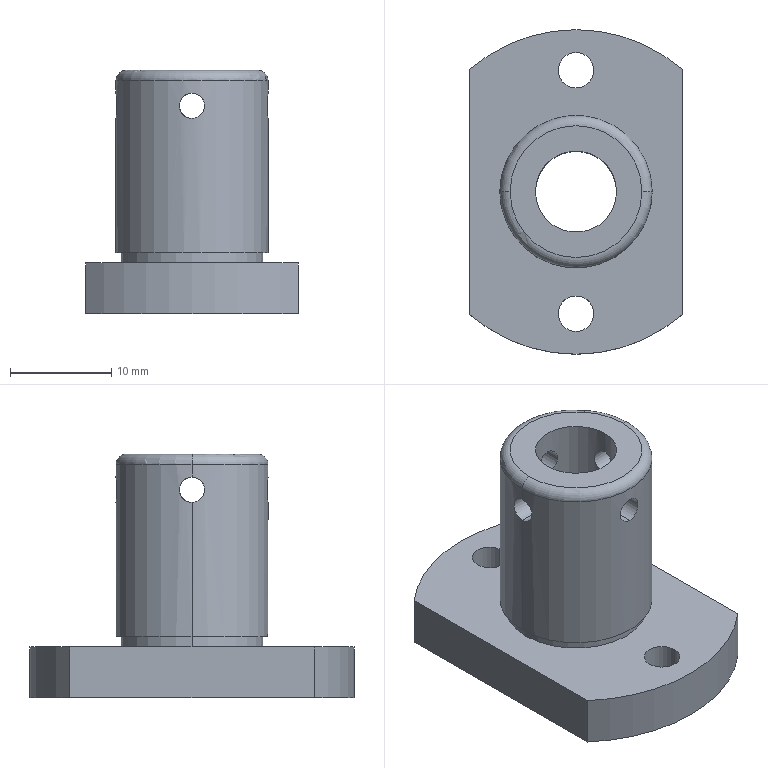Part | STEP file | 04-25 guide post mounting seat | 1 solid | 28 faces | box 21 x 32 x 24 mm | volume 5053 mm3 | cylinder 20 | plane 6 | torus 2 | commonest cylinder face diameters 2.5 x8 3.5 x4 8 x2 14 x2 15 x2 32 x2
STEP:
#1=CARTESIAN_POINT('',(-7.5,0.,21.75));
#2=VERTEX_POINT('',#1);
#3=CARTESIAN_POINT('',(-7.5,0.,19.25));
#4=VERTEX_POINT('',#3);
#5=CARTESIAN_POINT('',(-7.5,0.,21.75));
#6=CARTESIAN_POINT('',(-7.5,-0.1655,21.75));
#7=CARTESIAN_POINT('',(-7.494,-0.3279,21.717));
#8=CARTESIAN_POINT('',(-7.475,-0.6305,21.592));
#9=CARTESIAN_POINT('',(-7.461,-0.769,21.499));
#10=CARTESIAN_POINT('',(-7.434,-0.9992,21.269));
#11=CARTESIAN_POINT('',(-7.42,-1.092,21.129));
#12=CARTESIAN_POINT('',(-7.401,-1.217,20.829));
#13=CARTESIAN_POINT('',(-7.395,-1.25,20.664));
#14=CARTESIAN_POINT('',(-7.395,-1.25,20.419));
#15=CARTESIAN_POINT('',(-7.396,-1.242,20.336));
#16=CARTESIAN_POINT('',(-7.402,-1.21,20.175));
#17=CARTESIAN_POINT('',(-7.406,-1.186,20.097));
#18=CARTESIAN_POINT('',(-7.42,-1.092,19.87));
#19=CARTESIAN_POINT('',(-7.434,-1.,19.733));
#20=CARTESIAN_POINT('',(-7.462,-0.7675,19.5));
#21=CARTESIAN_POINT('',(-7.475,-0.6299,19.408));
#22=CARTESIAN_POINT('',(-7.49,-0.403,19.314));
#23=CARTESIAN_POINT('',(-7.493,-0.3251,19.29));
#24=CARTESIAN_POINT('',(-7.499,-0.1646,19.258));
#25=CARTESIAN_POINT('',(-7.5,-0.08166,19.25));
#26=CARTESIAN_POINT('',(-7.5,0.,19.25));
#27=B_SPLINE_CURVE_WITH_KNOTS('',3,(#5,#6,#7,#8,#9,#10,#11,#12,#13,#14,#15,#16,#17,#18,#19,#20,#21,#22,#23,#24,#25,#26),.UNSPECIFIED.,.F.,.F.,(4,2,2,2,2,2,2,2,2,2,4),(0.,0.0004894,0.0009787,0.001468,0.001957,0.002202,0.002447,0.002936,0.003426,0.00367,0.003915),.UNSPECIFIED.);
#28=EDGE_CURVE('',#2,#4,#27,.T.);
#29=ORIENTED_EDGE('',*,*,#28,.F.);
#30=CARTESIAN_POINT('',(-4.,0.,21.75));
#31=VERTEX_POINT('',#30);
#32=CARTESIAN_POINT('',(0.,0.,21.75));
#33=DIRECTION('',(1.,0.,0.));
#34=VECTOR('',#33,1000.);
#35=LINE('',#32,#34);
#36=EDGE_CURVE('',#2,#31,#35,.T.);
#37=ORIENTED_EDGE('',*,*,#36,.T.);
#38=CARTESIAN_POINT('',(-4.,0.,19.25));
#39=VERTEX_POINT('',#38);
#40=CARTESIAN_POINT('',(-4.,0.,21.75));
#41=CARTESIAN_POINT('',(-4.,-0.1663,21.75));
#42=CARTESIAN_POINT('',(-3.989,-0.3294,21.717));
#43=CARTESIAN_POINT('',(-3.953,-0.6318,21.591));
#44=CARTESIAN_POINT('',(-3.927,-0.7697,21.498));
#45=CARTESIAN_POINT('',(-3.875,-0.9987,21.269));
#46=CARTESIAN_POINT('',(-3.849,-1.092,21.13));
#47=CARTESIAN_POINT('',(-3.811,-1.217,20.83));
#48=CARTESIAN_POINT('',(-3.8,-1.25,20.665));
#49=CARTESIAN_POINT('',(-3.8,-1.25,20.418));
#50=CARTESIAN_POINT('',(-3.802,-1.242,20.335));
#51=CARTESIAN_POINT('',(-3.813,-1.21,20.174));
#52=CARTESIAN_POINT('',(-3.82,-1.186,20.096));
#53=CARTESIAN_POINT('',(-3.849,-1.091,19.868));
#54=CARTESIAN_POINT('',(-3.875,-0.9989,19.731));
#55=CARTESIAN_POINT('',(-3.914,-0.8259,19.558));
#56=CARTESIAN_POINT('',(-3.927,-0.7634,19.507));
#57=CARTESIAN_POINT('',(-3.951,-0.6283,19.416));
#58=CARTESIAN_POINT('',(-3.962,-0.5551,19.377));
#59=CARTESIAN_POINT('',(-3.989,-0.3291,19.283));
#60=CARTESIAN_POINT('',(-4.,-0.1639,19.25));
#61=CARTESIAN_POINT('',(-4.,0.,19.25));
#62=B_SPLINE_CURVE_WITH_KNOTS('',3,(#40,#41,#42,#43,#44,#45,#46,#47,#48,#49,#50,#51,#52,#53,#54,#55,#56,#57,#58,#59,#60,#61),.UNSPECIFIED.,.F.,.F.,(4,2,2,2,2,2,2,2,2,2,4),(0.,0.0004916,0.0009832,0.001475,0.001966,0.002212,0.002458,0.00295,0.003195,0.003441,0.003933),.UNSPECIFIED.);
#63=EDGE_CURVE('',#31,#39,#62,.T.);
#64=ORIENTED_EDGE('',*,*,#63,.T.);
#65=CARTESIAN_POINT('',(0.,0.,19.25));
#66=DIRECTION('',(1.,0.,0.));
#67=VECTOR('',#66,1000.);
#68=LINE('',#65,#67);
#69=EDGE_CURVE('',#4,#39,#68,.T.);
#70=ORIENTED_EDGE('',*,*,#69,.F.);
#71=EDGE_LOOP('',(#29,#37,#64,#70));
#72=FACE_OUTER_BOUND('',#71,.T.);
#73=CARTESIAN_POINT('',(0.,0.,20.5));
#74=DIRECTION('',(1.,0.,0.));
#75=DIRECTION('',(0.,0.,-1.));
#76=AXIS2_PLACEMENT_3D('',#73,#74,#75);
#77=CYLINDRICAL_SURFACE('',#76,1.25);
#78=ADVANCED_FACE('',(#72),#77,.F.);
#79=CARTESIAN_POINT('',(0.,-7.5,19.25));
#80=VERTEX_POINT('',#79);
#81=CARTESIAN_POINT('',(0.,-7.5,21.75));
#82=VERTEX_POINT('',#81);
#83=CARTESIAN_POINT('',(0.,-7.5,19.25));
#84=CARTESIAN_POINT('',(-0.1633,-7.5,19.25));
#85=CARTESIAN_POINT('',(-0.328,-7.494,19.283));
#86=CARTESIAN_POINT('',(-0.6289,-7.475,19.408));
#87=CARTESIAN_POINT('',(-0.768,-7.461,19.5));
#88=CARTESIAN_POINT('',(-0.941,-7.441,19.673));
#89=CARTESIAN_POINT('',(-0.9937,-7.434,19.737));
#90=CARTESIAN_POINT('',(-1.084,-7.421,19.873));
#91=CARTESIAN_POINT('',(-1.123,-7.416,19.944));
#92=CARTESIAN_POINT('',(-1.217,-7.401,20.172));
#93=CARTESIAN_POINT('',(-1.25,-7.395,20.334));
#94=CARTESIAN_POINT('',(-1.25,-7.395,20.664));
#95=CARTESIAN_POINT('',(-1.217,-7.401,20.827));
#96=CARTESIAN_POINT('',(-1.092,-7.42,21.129));
#97=CARTESIAN_POINT('',(-0.9994,-7.434,21.268));
#98=CARTESIAN_POINT('',(-0.7695,-7.461,21.498));
#99=CARTESIAN_POINT('',(-0.6304,-7.475,21.592));
#100=CARTESIAN_POINT('',(-0.3298,-7.494,21.717));
#101=CARTESIAN_POINT('',(-0.1655,-7.5,21.75));
#102=CARTESIAN_POINT('',(0.,-7.5,21.75));
#103=B_SPLINE_CURVE_WITH_KNOTS('',3,(#83,#84,#85,#86,#87,#88,#89,#90,#91,#92,#93,#94,#95,#96,#97,#98,#99,#100,#101,#102),.UNSPECIFIED.,.F.,.F.,(4,2,2,2,2,2,2,2,2,4),(0.003915,0.004404,0.004893,0.005138,0.005383,0.005872,0.006361,0.00685,0.00734,0.007829),.UNSPECIFIED.);
#104=EDGE_CURVE('',#80,#82,#103,.T.);
#105=ORIENTED_EDGE('',*,*,#104,.F.);
#106=CARTESIAN_POINT('',(0.,-4.,19.25));
#107=VERTEX_POINT('',#106);
#108=CARTESIAN_POINT('',(0.,0.,19.25));
#109=DIRECTION('',(0.,1.,0.));
#110=VECTOR('',#109,1000.);
#111=LINE('',#108,#110);
#112=EDGE_CURVE('',#80,#107,#111,.T.);
#113=ORIENTED_EDGE('',*,*,#112,.T.);
#114=CARTESIAN_POINT('',(0.,-4.,21.75));
#115=VERTEX_POINT('',#114);
#116=CARTESIAN_POINT('',(0.,-4.,19.25));
#117=CARTESIAN_POINT('',(-0.1638,-4.,19.25));
#118=CARTESIAN_POINT('',(-0.3292,-3.989,19.283));
#119=CARTESIAN_POINT('',(-0.6307,-3.953,19.408));
#120=CARTESIAN_POINT('',(-0.7685,-3.927,19.501));
#121=CARTESIAN_POINT('',(-0.9992,-3.875,19.731));
#122=CARTESIAN_POINT('',(-1.091,-3.849,19.868));
#123=CARTESIAN_POINT('',(-1.186,-3.82,20.096));
#124=CARTESIAN_POINT('',(-1.21,-3.813,20.174));
#125=CARTESIAN_POINT('',(-1.242,-3.802,20.334));
#126=CARTESIAN_POINT('',(-1.25,-3.8,20.418));
#127=CARTESIAN_POINT('',(-1.25,-3.8,20.665));
#128=CARTESIAN_POINT('',(-1.217,-3.811,20.829));
#129=CARTESIAN_POINT('',(-1.092,-3.849,21.131));
#130=CARTESIAN_POINT('',(-0.9987,-3.875,21.269));
#131=CARTESIAN_POINT('',(-0.7696,-3.927,21.498));
#132=CARTESIAN_POINT('',(-0.6317,-3.953,21.591));
#133=CARTESIAN_POINT('',(-0.3299,-3.989,21.717));
#134=CARTESIAN_POINT('',(-0.1663,-4.,21.75));
#135=CARTESIAN_POINT('',(0.,-4.,21.75));
#136=B_SPLINE_CURVE_WITH_KNOTS('',3,(#116,#117,#118,#119,#120,#121,#122,#123,#124,#125,#126,#127,#128,#129,#130,#131,#132,#133,#134,#135),.UNSPECIFIED.,.F.,.F.,(4,2,2,2,2,2,2,2,2,4),(0.003933,0.004424,0.004916,0.005407,0.005653,0.005899,0.00639,0.006882,0.007373,0.007865),.UNSPECIFIED.);
#137=EDGE_CURVE('',#107,#115,#136,.T.);
#138=ORIENTED_EDGE('',*,*,#137,.T.);
#139=CARTESIAN_POINT('',(0.,0.,21.75));
#140=DIRECTION('',(0.,1.,0.));
#141=VECTOR('',#140,1000.);
#142=LINE('',#139,#141);
#143=EDGE_CURVE('',#82,#115,#142,.T.);
#144=ORIENTED_EDGE('',*,*,#143,.F.);
#145=EDGE_LOOP('',(#105,#113,#138,#144));
#146=FACE_OUTER_BOUND('',#145,.T.);
#147=CARTESIAN_POINT('',(0.,0.,20.5));
#148=DIRECTION('',(0.,1.,0.));
#149=DIRECTION('',(0.,0.,1.));
#150=AXIS2_PLACEMENT_3D('',#147,#148,#149);
#151=CYLINDRICAL_SURFACE('',#150,1.25);
#152=ADVANCED_FACE('',(#146),#151,.F.);
#153=CARTESIAN_POINT('',(7.5,0.,19.25));
#154=VERTEX_POINT('',#153);
#155=CARTESIAN_POINT('',(7.5,0.,21.75));
#156=VERTEX_POINT('',#155);
#157=CARTESIAN_POINT('',(7.5,0.,19.25));
#158=CARTESIAN_POINT('',(7.5,-0.1633,19.25));
#159=CARTESIAN_POINT('',(7.494,-0.328,19.283));
#160=CARTESIAN_POINT('',(7.475,-0.6289,19.408));
#161=CARTESIAN_POINT('',(7.461,-0.768,19.5));
#162=CARTESIAN_POINT('',(7.441,-0.941,19.673));
#163=CARTESIAN_POINT('',(7.434,-0.9937,19.737));
#164=CARTESIAN_POINT('',(7.421,-1.084,19.873));
#165=CARTESIAN_POINT('',(7.416,-1.123,19.944));
#166=CARTESIAN_POINT('',(7.401,-1.217,20.172));
#167=CARTESIAN_POINT('',(7.395,-1.25,20.334));
#168=CARTESIAN_POINT('',(7.395,-1.25,20.664));
#169=CARTESIAN_POINT('',(7.401,-1.217,20.827));
#170=CARTESIAN_POINT('',(7.42,-1.092,21.129));
#171=CARTESIAN_POINT('',(7.434,-0.9994,21.268));
#172=CARTESIAN_POINT('',(7.461,-0.7695,21.498));
#173=CARTESIAN_POINT('',(7.475,-0.6304,21.592));
#174=CARTESIAN_POINT('',(7.494,-0.3298,21.717));
#175=CARTESIAN_POINT('',(7.5,-0.1655,21.75));
#176=CARTESIAN_POINT('',(7.5,0.,21.75));
#177=B_SPLINE_CURVE_WITH_KNOTS('',3,(#157,#158,#159,#160,#161,#162,#163,#164,#165,#166,#167,#168,#169,#170,#171,#172,#173,#174,#175,#176),.UNSPECIFIED.,.F.,.F.,(4,2,2,2,2,2,2,2,2,4),(0.003915,0.004404,0.004893,0.005138,0.005383,0.005872,0.006361,0.00685,0.00734,0.007829),.UNSPECIFIED.);
#178=EDGE_CURVE('',#154,#156,#177,.T.);
#179=ORIENTED_EDGE('',*,*,#178,.F.);
#180=CARTESIAN_POINT('',(4.,0.,19.25));
#181=VERTEX_POINT('',#180);
#182=CARTESIAN_POINT('',(0.,0.,19.25));
#183=DIRECTION('',(-1.,0.,0.));
#184=VECTOR('',#183,1000.);
#185=LINE('',#182,#184);
#186=EDGE_CURVE('',#154,#181,#185,.T.);
#187=ORIENTED_EDGE('',*,*,#186,.T.);
#188=CARTESIAN_POINT('',(4.,0.,21.75));
#189=VERTEX_POINT('',#188);
#190=CARTESIAN_POINT('',(4.,0.,19.25));
#191=CARTESIAN_POINT('',(4.,-0.1638,19.25));
#192=CARTESIAN_POINT('',(3.989,-0.3292,19.283));
#193=CARTESIAN_POINT('',(3.953,-0.6307,19.408));
#194=CARTESIAN_POINT('',(3.927,-0.7685,19.501));
#195=CARTESIAN_POINT('',(3.875,-0.9992,19.731));
#196=CARTESIAN_POINT('',(3.849,-1.091,19.868));
#197=CARTESIAN_POINT('',(3.82,-1.186,20.096));
#198=CARTESIAN_POINT('',(3.813,-1.21,20.174));
#199=CARTESIAN_POINT('',(3.802,-1.242,20.334));
#200=CARTESIAN_POINT('',(3.8,-1.25,20.418));
#201=CARTESIAN_POINT('',(3.8,-1.25,20.665));
#202=CARTESIAN_POINT('',(3.811,-1.217,20.829));
#203=CARTESIAN_POINT('',(3.849,-1.092,21.131));
#204=CARTESIAN_POINT('',(3.875,-0.9987,21.269));
#205=CARTESIAN_POINT('',(3.927,-0.7696,21.498));
#206=CARTESIAN_POINT('',(3.953,-0.6317,21.591));
#207=CARTESIAN_POINT('',(3.989,-0.3299,21.717));
#208=CARTESIAN_POINT('',(4.,-0.1663,21.75));
#209=CARTESIAN_POINT('',(4.,0.,21.75));
#210=B_SPLINE_CURVE_WITH_KNOTS('',3,(#190,#191,#192,#193,#194,#195,#196,#197,#198,#199,#200,#201,#202,#203,#204,#205,#206,#207,#208,#209),.UNSPECIFIED.,.F.,.F.,(4,2,2,2,2,2,2,2,2,4),(0.003933,0.004424,0.004916,0.005407,0.005653,0.005899,0.00639,0.006882,0.007373,0.007865),.UNSPECIFIED.);
#211=EDGE_CURVE('',#181,#189,#210,.T.);
#212=ORIENTED_EDGE('',*,*,#211,.T.);
#213=CARTESIAN_POINT('',(0.,0.,21.75));
#214=DIRECTION('',(-1.,0.,0.));
#215=VECTOR('',#214,1000.);
#216=LINE('',#213,#215);
#217=EDGE_CURVE('',#156,#189,#216,.T.);
#218=ORIENTED_EDGE('',*,*,#217,.F.);
#219=EDGE_LOOP('',(#179,#187,#212,#218));
#220=FACE_OUTER_BOUND('',#219,.T.);
#221=CARTESIAN_POINT('',(0.,0.,20.5));
#222=DIRECTION('',(-1.,0.,0.));
#223=DIRECTION('',(0.,0.,1.));
#224=AXIS2_PLACEMENT_3D('',#221,#222,#223);
#225=CYLINDRICAL_SURFACE('',#224,1.25);
#226=ADVANCED_FACE('',(#220),#225,.F.);
#227=CARTESIAN_POINT('',(0.,7.5,21.75));
#228=VERTEX_POINT('',#227);
#229=CARTESIAN_POINT('',(0.,7.5,19.25));
#230=VERTEX_POINT('',#229);
#231=CARTESIAN_POINT('',(0.,7.5,21.75));
#232=CARTESIAN_POINT('',(-0.1633,7.5,21.75));
#233=CARTESIAN_POINT('',(-0.328,7.494,21.717));
#234=CARTESIAN_POINT('',(-0.6289,7.475,21.592));
#235=CARTESIAN_POINT('',(-0.768,7.461,21.5));
#236=CARTESIAN_POINT('',(-0.941,7.441,21.327));
#237=CARTESIAN_POINT('',(-0.9937,7.434,21.263));
#238=CARTESIAN_POINT('',(-1.084,7.421,21.127));
#239=CARTESIAN_POINT('',(-1.123,7.416,21.056));
#240=CARTESIAN_POINT('',(-1.217,7.401,20.828));
#241=CARTESIAN_POINT('',(-1.25,7.395,20.666));
#242=CARTESIAN_POINT('',(-1.25,7.395,20.336));
#243=CARTESIAN_POINT('',(-1.217,7.401,20.173));
#244=CARTESIAN_POINT('',(-1.092,7.42,19.871));
#245=CARTESIAN_POINT('',(-0.9994,7.434,19.732));
#246=CARTESIAN_POINT('',(-0.7695,7.461,19.502));
#247=CARTESIAN_POINT('',(-0.6304,7.475,19.408));
#248=CARTESIAN_POINT('',(-0.3298,7.494,19.283));
#249=CARTESIAN_POINT('',(-0.1655,7.5,19.25));
#250=CARTESIAN_POINT('',(0.,7.5,19.25));
#251=B_SPLINE_CURVE_WITH_KNOTS('',3,(#231,#232,#233,#234,#235,#236,#237,#238,#239,#240,#241,#242,#243,#244,#245,#246,#247,#248,#249,#250),.UNSPECIFIED.,.F.,.F.,(4,2,2,2,2,2,2,2,2,4),(0.003915,0.004404,0.004893,0.005138,0.005383,0.005872,0.006361,0.00685,0.00734,0.007829),.UNSPECIFIED.);
#252=EDGE_CURVE('',#228,#230,#251,.T.);
#253=ORIENTED_EDGE('',*,*,#252,.F.);
#254=CARTESIAN_POINT('',(0.,4.,21.75));
#255=VERTEX_POINT('',#254);
#256=CARTESIAN_POINT('',(0.,0.,21.75));
#257=DIRECTION('',(0.,-1.,0.));
#258=VECTOR('',#257,1000.);
#259=LINE('',#256,#258);
#260=EDGE_CURVE('',#228,#255,#259,.T.);
#261=ORIENTED_EDGE('',*,*,#260,.T.);
#262=CARTESIAN_POINT('',(0.,4.,19.25));
#263=VERTEX_POINT('',#262);
#264=CARTESIAN_POINT('',(0.,4.,21.75));
#265=CARTESIAN_POINT('',(-0.1638,4.,21.75));
#266=CARTESIAN_POINT('',(-0.3292,3.989,21.717));
#267=CARTESIAN_POINT('',(-0.6307,3.953,21.592));
#268=CARTESIAN_POINT('',(-0.7685,3.927,21.499));
#269=CARTESIAN_POINT('',(-0.9992,3.875,21.269));
#270=CARTESIAN_POINT('',(-1.091,3.849,21.132));
#271=CARTESIAN_POINT('',(-1.186,3.82,20.904));
#272=CARTESIAN_POINT('',(-1.21,3.813,20.826));
#273=CARTESIAN_POINT('',(-1.242,3.802,20.666));
#274=CARTESIAN_POINT('',(-1.25,3.8,20.582));
#275=CARTESIAN_POINT('',(-1.25,3.8,20.335));
#276=CARTESIAN_POINT('',(-1.217,3.811,20.171));
#277=CARTESIAN_POINT('',(-1.092,3.849,19.869));
#278=CARTESIAN_POINT('',(-0.9987,3.875,19.731));
#279=CARTESIAN_POINT('',(-0.7696,3.927,19.502));
#280=CARTESIAN_POINT('',(-0.6317,3.953,19.409));
#281=CARTESIAN_POINT('',(-0.3299,3.989,19.283));
#282=CARTESIAN_POINT('',(-0.1663,4.,19.25));
#283=CARTESIAN_POINT('',(0.,4.,19.25));
#284=B_SPLINE_CURVE_WITH_KNOTS('',3,(#264,#265,#266,#267,#268,#269,#270,#271,#272,#273,#274,#275,#276,#277,#278,#279,#280,#281,#282,#283),.UNSPECIFIED.,.F.,.F.,(4,2,2,2,2,2,2,2,2,4),(0.003933,0.004424,0.004916,0.005407,0.005653,0.005899,0.00639,0.006882,0.007373,0.007865),.UNSPECIFIED.);
#285=EDGE_CURVE('',#255,#263,#284,.T.);
#286=ORIENTED_EDGE('',*,*,#285,.T.);
#287=CARTESIAN_POINT('',(0.,0.,19.25));
#288=DIRECTION('',(0.,-1.,0.));
#289=VECTOR('',#288,1000.);
#290=LINE('',#287,#289);
#291=EDGE_CURVE('',#230,#263,#290,.T.);
#292=ORIENTED_EDGE('',*,*,#291,.F.);
#293=EDGE_LOOP('',(#253,#261,#286,#292));
#294=FACE_OUTER_BOUND('',#293,.T.);
#295=CARTESIAN_POINT('',(0.,0.,20.5));
#296=DIRECTION('',(0.,-1.,0.));
#297=DIRECTION('',(0.,0.,-1.));
#298=AXIS2_PLACEMENT_3D('',#295,#296,#297);
#299=CYLINDRICAL_SURFACE('',#298,1.25);
#300=ADVANCED_FACE('',(#294),#299,.F.);
#301=CARTESIAN_POINT('',(7.,0.,6.));
#302=VERTEX_POINT('',#301);
#303=CARTESIAN_POINT('',(-7.,0.,6.));
#304=VERTEX_POINT('',#303);
#305=CARTESIAN_POINT('',(0.,0.,6.));
#306=DIRECTION('',(0.,0.,1.));
#307=DIRECTION('',(1.,0.,0.));
#308=AXIS2_PLACEMENT_3D('',#305,#306,#307);
#309=CIRCLE('',#308,7.);
#310=EDGE_CURVE('',#302,#304,#309,.T.);
#311=ORIENTED_EDGE('',*,*,#310,.F.);
#312=CARTESIAN_POINT('',(7.,0.,5.));
#313=VERTEX_POINT('',#312);
#314=CARTESIAN_POINT('',(7.,0.,6.));
#315=DIRECTION('',(0.,0.,-1.));
#316=VECTOR('',#315,1000.);
#317=LINE('',#314,#316);
#318=EDGE_CURVE('',#302,#313,#317,.T.);
#319=ORIENTED_EDGE('',*,*,#318,.T.);
#320=CARTESIAN_POINT('',(-7.,0.,5.));
#321=VERTEX_POINT('',#320);
#322=CARTESIAN_POINT('',(0.,0.,5.));
#323=DIRECTION('',(0.,0.,1.));
#324=DIRECTION('',(1.,0.,0.));
#325=AXIS2_PLACEMENT_3D('',#322,#323,#324);
#326=CIRCLE('',#325,7.);
#327=EDGE_CURVE('',#313,#321,#326,.T.);
#328=ORIENTED_EDGE('',*,*,#327,.T.);
#329=CARTESIAN_POINT('',(-7.,0.,6.));
#330=DIRECTION('',(0.,0.,-1.));
#331=VECTOR('',#330,1000.);
#332=LINE('',#329,#331);
#333=EDGE_CURVE('',#304,#321,#332,.T.);
#334=ORIENTED_EDGE('',*,*,#333,.F.);
#335=EDGE_LOOP('',(#311,#319,#328,#334));
#336=FACE_OUTER_BOUND('',#335,.T.);
#337=CARTESIAN_POINT('',(0.,0.,6.));
#338=DIRECTION('',(0.,0.,-1.));
#339=DIRECTION('',(-1.,0.,0.));
#340=AXIS2_PLACEMENT_3D('',#337,#338,#339);
#341=CYLINDRICAL_SURFACE('',#340,7.);
#342=ADVANCED_FACE('',(#336),#341,.T.);
#343=CARTESIAN_POINT('',(-7.5,0.,23.));
#344=VERTEX_POINT('',#343);
#345=CARTESIAN_POINT('',(7.5,0.,23.));
#346=VERTEX_POINT('',#345);
#347=CARTESIAN_POINT('',(0.,0.,23.));
#348=DIRECTION('',(0.,0.,-1.));
#349=DIRECTION('',(1.,0.,0.));
#350=AXIS2_PLACEMENT_3D('',#347,#348,#349);
#351=CIRCLE('',#350,7.5);
#352=EDGE_CURVE('',#344,#346,#351,.T.);
#353=ORIENTED_EDGE('',*,*,#352,.F.);
#354=CARTESIAN_POINT('',(-6.5,0.,24.));
#355=VERTEX_POINT('',#354);
#356=CARTESIAN_POINT('',(-6.5,0.,23.));
#357=DIRECTION('',(0.,1.,0.));
#358=DIRECTION('',(-1.,0.,0.));
#359=AXIS2_PLACEMENT_3D('',#356,#357,#358);
#360=CIRCLE('',#359,1.);
#361=EDGE_CURVE('',#344,#355,#360,.T.);
#362=ORIENTED_EDGE('',*,*,#361,.T.);
#363=CARTESIAN_POINT('',(6.5,0.,24.));
#364=VERTEX_POINT('',#363);
#365=CARTESIAN_POINT('',(0.,0.,24.));
#366=DIRECTION('',(0.,0.,1.));
#367=DIRECTION('',(1.,0.,0.));
#368=AXIS2_PLACEMENT_3D('',#365,#366,#367);
#369=CIRCLE('',#368,6.5);
#370=EDGE_CURVE('',#364,#355,#369,.T.);
#371=ORIENTED_EDGE('',*,*,#370,.F.);
#372=CARTESIAN_POINT('',(6.5,0.,23.));
#373=DIRECTION('',(0.,-1.,0.));
#374=DIRECTION('',(0.,0.,-1.));
#375=AXIS2_PLACEMENT_3D('',#372,#373,#374);
#376=CIRCLE('',#375,1.);
#377=EDGE_CURVE('',#346,#364,#376,.T.);
#378=ORIENTED_EDGE('',*,*,#377,.F.);
#379=EDGE_LOOP('',(#353,#362,#371,#378));
#380=FACE_OUTER_BOUND('',#379,.T.);
#381=CARTESIAN_POINT('',(0.,0.,23.));
#382=DIRECTION('',(0.,0.,1.));
#383=DIRECTION('',(1.,0.,0.));
#384=AXIS2_PLACEMENT_3D('',#381,#382,#383);
#385=TOROIDAL_SURFACE('',#384,6.5,1.);
#386=ADVANCED_FACE('',(#380),#385,.T.);
#387=CARTESIAN_POINT('',(1.75,-12.,5.));
#388=VERTEX_POINT('',#387);
#389=CARTESIAN_POINT('',(-1.75,-12.,5.));
#390=VERTEX_POINT('',#389);
#391=CARTESIAN_POINT('',(0.,-12.,5.));
#392=DIRECTION('',(0.,0.,-1.));
#393=DIRECTION('',(-1.,0.,0.));
#394=AXIS2_PLACEMENT_3D('',#391,#392,#393);
#395=CIRCLE('',#394,1.75);
#396=EDGE_CURVE('',#388,#390,#395,.T.);
#397=ORIENTED_EDGE('',*,*,#396,.F.);
#398=CARTESIAN_POINT('',(1.75,-12.,0.));
#399=VERTEX_POINT('',#398);
#400=CARTESIAN_POINT('',(1.75,-12.,10.));
#401=DIRECTION('',(0.,0.,-1.));
#402=VECTOR('',#401,1000.);
#403=LINE('',#400,#402);
#404=EDGE_CURVE('',#388,#399,#403,.T.);
#405=ORIENTED_EDGE('',*,*,#404,.T.);
#406=CARTESIAN_POINT('',(-1.75,-12.,0.));
#407=VERTEX_POINT('',#406);
#408=CARTESIAN_POINT('',(0.,-12.,0.));
#409=DIRECTION('',(0.,0.,-1.));
#410=DIRECTION('',(-1.,0.,0.));
#411=AXIS2_PLACEMENT_3D('',#408,#409,#410);
#412=CIRCLE('',#411,1.75);
#413=EDGE_CURVE('',#399,#407,#412,.T.);
#414=ORIENTED_EDGE('',*,*,#413,.T.);
#415=CARTESIAN_POINT('',(-1.75,-12.,10.));
#416=DIRECTION('',(0.,0.,-1.));
#417=VECTOR('',#416,1000.);
#418=LINE('',#415,#417);
#419=EDGE_CURVE('',#390,#407,#418,.T.);
#420=ORIENTED_EDGE('',*,*,#419,.F.);
#421=EDGE_LOOP('',(#397,#405,#414,#420));
#422=FACE_OUTER_BOUND('',#421,.T.);
#423=CARTESIAN_POINT('',(0.,-12.,10.));
#424=DIRECTION('',(0.,0.,-1.));
#425=DIRECTION('',(-1.,0.,0.));
#426=AXIS2_PLACEMENT_3D('',#423,#424,#425);
#427=CYLINDRICAL_SURFACE('',#426,1.75);
#428=ADVANCED_FACE('',(#422),#427,.F.);
#429=CARTESIAN_POINT('',(1.75,12.,5.));
#430=VERTEX_POINT('',#429);
#431=CARTESIAN_POINT('',(-1.75,12.,5.));
#432=VERTEX_POINT('',#431);
#433=CARTESIAN_POINT('',(0.,12.,5.));
#434=DIRECTION('',(0.,0.,-1.));
#435=DIRECTION('',(-1.,0.,0.));
#436=AXIS2_PLACEMENT_3D('',#433,#434,#435);
#437=CIRCLE('',#436,1.75);
#438=EDGE_CURVE('',#430,#432,#437,.T.);
#439=ORIENTED_EDGE('',*,*,#438,.F.);
#440=CARTESIAN_POINT('',(1.75,12.,0.));
#441=VERTEX_POINT('',#440);
#442=CARTESIAN_POINT('',(1.75,12.,10.));
#443=DIRECTION('',(0.,0.,-1.));
#444=VECTOR('',#443,1000.);
#445=LINE('',#442,#444);
#446=EDGE_CURVE('',#430,#441,#445,.T.);
#447=ORIENTED_EDGE('',*,*,#446,.T.);
#448=CARTESIAN_POINT('',(-1.75,12.,0.));
#449=VERTEX_POINT('',#448);
#450=CARTESIAN_POINT('',(0.,12.,0.));
#451=DIRECTION('',(0.,0.,-1.));
#452=DIRECTION('',(-1.,0.,0.));
#453=AXIS2_PLACEMENT_3D('',#450,#451,#452);
#454=CIRCLE('',#453,1.75);
#455=EDGE_CURVE('',#441,#449,#454,.T.);
#456=ORIENTED_EDGE('',*,*,#455,.T.);
#457=CARTESIAN_POINT('',(-1.75,12.,10.));
#458=DIRECTION('',(0.,0.,-1.));
#459=VECTOR('',#458,1000.);
#460=LINE('',#457,#459);
#461=EDGE_CURVE('',#432,#449,#460,.T.);
#462=ORIENTED_EDGE('',*,*,#461,.F.);
#463=EDGE_LOOP('',(#439,#447,#456,#462));
#464=FACE_OUTER_BOUND('',#463,.T.);
#465=CARTESIAN_POINT('',(0.,12.,10.));
#466=DIRECTION('',(0.,0.,-1.));
#467=DIRECTION('',(-1.,0.,0.));
#468=AXIS2_PLACEMENT_3D('',#465,#466,#467);
#469=CYLINDRICAL_SURFACE('',#468,1.75);
#470=ADVANCED_FACE('',(#464),#469,.F.);
#471=CARTESIAN_POINT('',(0.,-4.,21.75));
#472=CARTESIAN_POINT('',(0.1663,-4.,21.75));
#473=CARTESIAN_POINT('',(0.3294,-3.989,21.717));
#474=CARTESIAN_POINT('',(0.6318,-3.953,21.591));
#475=CARTESIAN_POINT('',(0.7697,-3.927,21.498));
#476=CARTESIAN_POINT('',(0.9987,-3.875,21.269));
#477=CARTESIAN_POINT('',(1.092,-3.849,21.13));
#478=CARTESIAN_POINT('',(1.217,-3.811,20.83));
#479=CARTESIAN_POINT('',(1.25,-3.8,20.665));
#480=CARTESIAN_POINT('',(1.25,-3.8,20.418));
#481=CARTESIAN_POINT('',(1.242,-3.802,20.335));
#482=CARTESIAN_POINT('',(1.21,-3.813,20.174));
#483=CARTESIAN_POINT('',(1.186,-3.82,20.096));
#484=CARTESIAN_POINT('',(1.091,-3.849,19.868));
#485=CARTESIAN_POINT('',(0.9989,-3.875,19.731));
#486=CARTESIAN_POINT('',(0.8259,-3.914,19.558));
#487=CARTESIAN_POINT('',(0.7634,-3.927,19.507));
#488=CARTESIAN_POINT('',(0.6283,-3.951,19.416));
#489=CARTESIAN_POINT('',(0.5551,-3.962,19.377));
#490=CARTESIAN_POINT('',(0.3291,-3.989,19.283));
#491=CARTESIAN_POINT('',(0.1639,-4.,19.25));
#492=CARTESIAN_POINT('',(0.,-4.,19.25));
#493=B_SPLINE_CURVE_WITH_KNOTS('',3,(#471,#472,#473,#474,#475,#476,#477,#478,#479,#480,#481,#482,#483,#484,#485,#486,#487,#488,#489,#490,#491,#492),.UNSPECIFIED.,.F.,.F.,(4,2,2,2,2,2,2,2,2,2,4),(0.,0.0004916,0.0009832,0.001475,0.001966,0.002212,0.002458,0.00295,0.003195,0.003441,0.003933),.UNSPECIFIED.);
#494=EDGE_CURVE('',#115,#107,#493,.T.);
#495=ORIENTED_EDGE('',*,*,#494,.F.);
#496=ORIENTED_EDGE('',*,*,#137,.F.);
#497=EDGE_LOOP('',(#495,#496));
#498=FACE_BOUND('',#497,.T.);
#499=CARTESIAN_POINT('',(-4.,0.,24.));
#500=VERTEX_POINT('',#499);
#501=CARTESIAN_POINT('',(4.,0.,24.));
#502=VERTEX_POINT('',#501);
#503=CARTESIAN_POINT('',(0.,0.,24.));
#504=DIRECTION('',(0.,0.,1.));
#505=DIRECTION('',(1.,0.,0.));
#506=AXIS2_PLACEMENT_3D('',#503,#504,#505);
#507=CIRCLE('',#506,4.);
#508=EDGE_CURVE('',#500,#502,#507,.T.);
#509=ORIENTED_EDGE('',*,*,#508,.T.);
#510=CARTESIAN_POINT('',(4.,0.,24.));
#511=DIRECTION('',(0.,0.,-1.));
#512=VECTOR('',#511,1000.);
#513=LINE('',#510,#512);
#514=EDGE_CURVE('',#502,#189,#513,.T.);
#515=ORIENTED_EDGE('',*,*,#514,.T.);
#516=ORIENTED_EDGE('',*,*,#211,.F.);
#517=CARTESIAN_POINT('',(4.,0.,0.));
#518=VERTEX_POINT('',#517);
#519=CARTESIAN_POINT('',(4.,0.,24.));
#520=DIRECTION('',(0.,0.,-1.));
#521=VECTOR('',#520,1000.);
#522=LINE('',#519,#521);
#523=EDGE_CURVE('',#181,#518,#522,.T.);
#524=ORIENTED_EDGE('',*,*,#523,.T.);
#525=CARTESIAN_POINT('',(-4.,0.,0.));
#526=VERTEX_POINT('',#525);
#527=CARTESIAN_POINT('',(0.,0.,0.));
#528=DIRECTION('',(0.,0.,1.));
#529=DIRECTION('',(1.,0.,0.));
#530=AXIS2_PLACEMENT_3D('',#527,#528,#529);
#531=CIRCLE('',#530,4.);
#532=EDGE_CURVE('',#526,#518,#531,.T.);
#533=ORIENTED_EDGE('',*,*,#532,.F.);
#534=CARTESIAN_POINT('',(-4.,0.,24.));
#535=DIRECTION('',(0.,0.,-1.));
#536=VECTOR('',#535,1000.);
#537=LINE('',#534,#536);
#538=EDGE_CURVE('',#39,#526,#537,.T.);
#539=ORIENTED_EDGE('',*,*,#538,.F.);
#540=ORIENTED_EDGE('',*,*,#63,.F.);
#541=CARTESIAN_POINT('',(-4.,0.,24.));
#542=DIRECTION('',(0.,0.,-1.));
#543=VECTOR('',#542,1000.);
#544=LINE('',#541,#543);
#545=EDGE_CURVE('',#500,#31,#544,.T.);
#546=ORIENTED_EDGE('',*,*,#545,.F.);
#547=EDGE_LOOP('',(#509,#515,#516,#524,#533,#539,#540,#546));
#548=FACE_OUTER_BOUND('',#547,.T.);
#549=CARTESIAN_POINT('',(0.,0.,24.));
#550=DIRECTION('',(0.,0.,-1.));
#551=DIRECTION('',(-1.,0.,0.));
#552=AXIS2_PLACEMENT_3D('',#549,#550,#551);
#553=CYLINDRICAL_SURFACE('',#552,4.);
#554=ADVANCED_FACE('',(#498,#548),#553,.F.);
#555=CARTESIAN_POINT('',(0.,7.5,19.25));
#556=CARTESIAN_POINT('',(0.1655,7.5,19.25));
#557=CARTESIAN_POINT('',(0.3279,7.494,19.283));
#558=CARTESIAN_POINT('',(0.6305,7.475,19.408));
#559=CARTESIAN_POINT('',(0.769,7.461,19.501));
#560=CARTESIAN_POINT('',(0.9992,7.434,19.731));
#561=CARTESIAN_POINT('',(1.092,7.42,19.871));
#562=CARTESIAN_POINT('',(1.217,7.401,20.171));
#563=CARTESIAN_POINT('',(1.25,7.395,20.336));
#564=CARTESIAN_POINT('',(1.25,7.395,20.581));
#565=CARTESIAN_POINT('',(1.242,7.396,20.664));
#566=CARTESIAN_POINT('',(1.21,7.402,20.825));
#567=CARTESIAN_POINT('',(1.186,7.406,20.903));
#568=CARTESIAN_POINT('',(1.092,7.42,21.13));
#569=CARTESIAN_POINT('',(1.,7.434,21.267));
#570=CARTESIAN_POINT('',(0.7675,7.462,21.5));
#571=CARTESIAN_POINT('',(0.6299,7.475,21.592));
#572=CARTESIAN_POINT('',(0.403,7.49,21.686));
#573=CARTESIAN_POINT('',(0.3251,7.493,21.71));
#574=CARTESIAN_POINT('',(0.1646,7.499,21.742));
#575=CARTESIAN_POINT('',(0.08166,7.5,21.75));
#576=CARTESIAN_POINT('',(0.,7.5,21.75));
#577=B_SPLINE_CURVE_WITH_KNOTS('',3,(#555,#556,#557,#558,#559,#560,#561,#562,#563,#564,#565,#566,#567,#568,#569,#570,#571,#572,#573,#574,#575,#576),.UNSPECIFIED.,.F.,.F.,(4,2,2,2,2,2,2,2,2,2,4),(0.,0.0004894,0.0009787,0.001468,0.001957,0.002202,0.002447,0.002936,0.003426,0.00367,0.003915),.UNSPECIFIED.);
#578=EDGE_CURVE('',#230,#228,#577,.T.);
#579=ORIENTED_EDGE('',*,*,#578,.T.);
#580=ORIENTED_EDGE('',*,*,#252,.T.);
#581=EDGE_LOOP('',(#579,#580));
#582=FACE_BOUND('',#581,.T.);
#583=ORIENTED_EDGE('',*,*,#352,.T.);
#584=CARTESIAN_POINT('',(7.5,0.,24.));
#585=DIRECTION('',(0.,0.,-1.));
#586=VECTOR('',#585,1000.);
#587=LINE('',#584,#586);
#588=EDGE_CURVE('',#346,#156,#587,.T.);
#589=ORIENTED_EDGE('',*,*,#588,.T.);
#590=CARTESIAN_POINT('',(7.5,0.,21.75));
#591=CARTESIAN_POINT('',(7.5,0.1655,21.75));
#592=CARTESIAN_POINT('',(7.494,0.3279,21.717));
#593=CARTESIAN_POINT('',(7.475,0.6305,21.592));
#594=CARTESIAN_POINT('',(7.461,0.769,21.499));
#595=CARTESIAN_POINT('',(7.434,0.9992,21.269));
#596=CARTESIAN_POINT('',(7.42,1.092,21.129));
#597=CARTESIAN_POINT('',(7.401,1.217,20.829));
#598=CARTESIAN_POINT('',(7.395,1.25,20.664));
#599=CARTESIAN_POINT('',(7.395,1.25,20.419));
#600=CARTESIAN_POINT('',(7.396,1.242,20.336));
#601=CARTESIAN_POINT('',(7.402,1.21,20.175));
#602=CARTESIAN_POINT('',(7.406,1.186,20.097));
#603=CARTESIAN_POINT('',(7.42,1.092,19.87));
#604=CARTESIAN_POINT('',(7.434,1.,19.733));
#605=CARTESIAN_POINT('',(7.462,0.7675,19.5));
#606=CARTESIAN_POINT('',(7.475,0.6299,19.408));
#607=CARTESIAN_POINT('',(7.49,0.403,19.314));
#608=CARTESIAN_POINT('',(7.493,0.3251,19.29));
#609=CARTESIAN_POINT('',(7.499,0.1646,19.258));
#610=CARTESIAN_POINT('',(7.5,0.08166,19.25));
#611=CARTESIAN_POINT('',(7.5,0.,19.25));
#612=B_SPLINE_CURVE_WITH_KNOTS('',3,(#590,#591,#592,#593,#594,#595,#596,#597,#598,#599,#600,#601,#602,#603,#604,#605,#606,#607,#608,#609,#610,#611),.UNSPECIFIED.,.F.,.F.,(4,2,2,2,2,2,2,2,2,2,4),(0.,0.0004894,0.0009787,0.001468,0.001957,0.002202,0.002447,0.002936,0.003426,0.00367,0.003915),.UNSPECIFIED.);
#613=EDGE_CURVE('',#156,#154,#612,.T.);
#614=ORIENTED_EDGE('',*,*,#613,.T.);
#615=CARTESIAN_POINT('',(7.5,0.,6.));
#616=VERTEX_POINT('',#615);
#617=CARTESIAN_POINT('',(7.5,0.,24.));
#618=DIRECTION('',(0.,0.,-1.));
#619=VECTOR('',#618,1000.);
#620=LINE('',#617,#619);
#621=EDGE_CURVE('',#154,#616,#620,.T.);
#622=ORIENTED_EDGE('',*,*,#621,.T.);
#623=CARTESIAN_POINT('',(-7.5,0.,6.));
#624=VERTEX_POINT('',#623);
#625=CARTESIAN_POINT('',(0.,0.,6.));
#626=DIRECTION('',(0.,0.,1.));
#627=DIRECTION('',(1.,0.,0.));
#628=AXIS2_PLACEMENT_3D('',#625,#626,#627);
#629=CIRCLE('',#628,7.5);
#630=EDGE_CURVE('',#616,#624,#629,.T.);
#631=ORIENTED_EDGE('',*,*,#630,.T.);
#632=CARTESIAN_POINT('',(-7.5,0.,24.));
#633=DIRECTION('',(0.,0.,-1.));
#634=VECTOR('',#633,1000.);
#635=LINE('',#632,#634);
#636=EDGE_CURVE('',#4,#624,#635,.T.);
#637=ORIENTED_EDGE('',*,*,#636,.F.);
#638=CARTESIAN_POINT('',(-7.5,0.,19.25));
#639=CARTESIAN_POINT('',(-7.5,0.1633,19.25));
#640=CARTESIAN_POINT('',(-7.494,0.328,19.283));
#641=CARTESIAN_POINT('',(-7.475,0.6289,19.408));
#642=CARTESIAN_POINT('',(-7.461,0.768,19.5));
#643=CARTESIAN_POINT('',(-7.441,0.941,19.673));
#644=CARTESIAN_POINT('',(-7.434,0.9937,19.737));
#645=CARTESIAN_POINT('',(-7.421,1.084,19.873));
#646=CARTESIAN_POINT('',(-7.416,1.123,19.944));
#647=CARTESIAN_POINT('',(-7.401,1.217,20.172));
#648=CARTESIAN_POINT('',(-7.395,1.25,20.334));
#649=CARTESIAN_POINT('',(-7.395,1.25,20.664));
#650=CARTESIAN_POINT('',(-7.401,1.217,20.827));
#651=CARTESIAN_POINT('',(-7.42,1.092,21.129));
#652=CARTESIAN_POINT('',(-7.434,0.9994,21.268));
#653=CARTESIAN_POINT('',(-7.461,0.7695,21.498));
#654=CARTESIAN_POINT('',(-7.475,0.6304,21.592));
#655=CARTESIAN_POINT('',(-7.494,0.3298,21.717));
#656=CARTESIAN_POINT('',(-7.5,0.1655,21.75));
#657=CARTESIAN_POINT('',(-7.5,0.,21.75));
#658=B_SPLINE_CURVE_WITH_KNOTS('',3,(#638,#639,#640,#641,#642,#643,#644,#645,#646,#647,#648,#649,#650,#651,#652,#653,#654,#655,#656,#657),.UNSPECIFIED.,.F.,.F.,(4,2,2,2,2,2,2,2,2,4),(0.003915,0.004404,0.004893,0.005138,0.005383,0.005872,0.006361,0.00685,0.00734,0.007829),.UNSPECIFIED.);
#659=EDGE_CURVE('',#4,#2,#658,.T.);
#660=ORIENTED_EDGE('',*,*,#659,.T.);
#661=CARTESIAN_POINT('',(-7.5,0.,24.));
#662=DIRECTION('',(0.,0.,-1.));
#663=VECTOR('',#662,1000.);
#664=LINE('',#661,#663);
#665=EDGE_CURVE('',#344,#2,#664,.T.);
#666=ORIENTED_EDGE('',*,*,#665,.F.);
#667=EDGE_LOOP('',(#583,#589,#614,#622,#631,#637,#660,#666));
#668=FACE_OUTER_BOUND('',#667,.T.);
#669=CARTESIAN_POINT('',(0.,0.,24.));
#670=DIRECTION('',(0.,0.,-1.));
#671=DIRECTION('',(-1.,0.,0.));
#672=AXIS2_PLACEMENT_3D('',#669,#670,#671);
#673=CYLINDRICAL_SURFACE('',#672,7.5);
#674=ADVANCED_FACE('',(#582,#668),#673,.T.);
#675=ORIENTED_EDGE('',*,*,#588,.F.);
#676=CARTESIAN_POINT('',(0.,0.,23.));
#677=DIRECTION('',(0.,0.,-1.));
#678=DIRECTION('',(1.,0.,0.));
#679=AXIS2_PLACEMENT_3D('',#676,#677,#678);
#680=CIRCLE('',#679,7.5);
#681=EDGE_CURVE('',#346,#344,#680,.T.);
#682=ORIENTED_EDGE('',*,*,#681,.T.);
#683=ORIENTED_EDGE('',*,*,#665,.T.);
#684=ORIENTED_EDGE('',*,*,#28,.T.);
#685=ORIENTED_EDGE('',*,*,#636,.T.);
#686=CARTESIAN_POINT('',(0.,0.,6.));
#687=DIRECTION('',(0.,0.,1.));
#688=DIRECTION('',(1.,0.,0.));
#689=AXIS2_PLACEMENT_3D('',#686,#687,#688);
#690=CIRCLE('',#689,7.5);
#691=EDGE_CURVE('',#624,#616,#690,.T.);
#692=ORIENTED_EDGE('',*,*,#691,.T.);
#693=ORIENTED_EDGE('',*,*,#621,.F.);
#694=ORIENTED_EDGE('',*,*,#178,.T.);
#695=EDGE_LOOP('',(#675,#682,#683,#684,#685,#692,#693,#694));
#696=FACE_OUTER_BOUND('',#695,.T.);
#697=CARTESIAN_POINT('',(0.,-7.5,21.75));
#698=CARTESIAN_POINT('',(0.1655,-7.5,21.75));
#699=CARTESIAN_POINT('',(0.3279,-7.494,21.717));
#700=CARTESIAN_POINT('',(0.6305,-7.475,21.592));
#701=CARTESIAN_POINT('',(0.769,-7.461,21.499));
#702=CARTESIAN_POINT('',(0.9992,-7.434,21.269));
#703=CARTESIAN_POINT('',(1.092,-7.42,21.129));
#704=CARTESIAN_POINT('',(1.217,-7.401,20.829));
#705=CARTESIAN_POINT('',(1.25,-7.395,20.664));
#706=CARTESIAN_POINT('',(1.25,-7.395,20.419));
#707=CARTESIAN_POINT('',(1.242,-7.396,20.336));
#708=CARTESIAN_POINT('',(1.21,-7.402,20.175));
#709=CARTESIAN_POINT('',(1.186,-7.406,20.097));
#710=CARTESIAN_POINT('',(1.092,-7.42,19.87));
#711=CARTESIAN_POINT('',(1.,-7.434,19.733));
#712=CARTESIAN_POINT('',(0.7675,-7.462,19.5));
#713=CARTESIAN_POINT('',(0.6299,-7.475,19.408));
#714=CARTESIAN_POINT('',(0.403,-7.49,19.314));
#715=CARTESIAN_POINT('',(0.3251,-7.493,19.29));
#716=CARTESIAN_POINT('',(0.1646,-7.499,19.258));
#717=CARTESIAN_POINT('',(0.08166,-7.5,19.25));
#718=CARTESIAN_POINT('',(0.,-7.5,19.25));
#719=B_SPLINE_CURVE_WITH_KNOTS('',3,(#697,#698,#699,#700,#701,#702,#703,#704,#705,#706,#707,#708,#709,#710,#711,#712,#713,#714,#715,#716,#717,#718),.UNSPECIFIED.,.F.,.F.,(4,2,2,2,2,2,2,2,2,2,4),(0.,0.0004894,0.0009787,0.001468,0.001957,0.002202,0.002447,0.002936,0.003426,0.00367,0.003915),.UNSPECIFIED.);
#720=EDGE_CURVE('',#82,#80,#719,.T.);
#721=ORIENTED_EDGE('',*,*,#720,.T.);
#722=ORIENTED_EDGE('',*,*,#104,.T.);
#723=EDGE_LOOP('',(#721,#722));
#724=FACE_BOUND('',#723,.T.);
#725=CARTESIAN_POINT('',(0.,0.,24.));
#726=DIRECTION('',(0.,0.,-1.));
#727=DIRECTION('',(-1.,0.,0.));
#728=AXIS2_PLACEMENT_3D('',#725,#726,#727);
#729=CYLINDRICAL_SURFACE('',#728,7.5);
#730=ADVANCED_FACE('',(#696,#724),#729,.T.);
#731=ORIENTED_EDGE('',*,*,#370,.T.);
#732=CARTESIAN_POINT('',(0.,0.,24.));
#733=DIRECTION('',(0.,0.,1.));
#734=DIRECTION('',(1.,0.,0.));
#735=AXIS2_PLACEMENT_3D('',#732,#733,#734);
#736=CIRCLE('',#735,6.5);
#737=EDGE_CURVE('',#355,#364,#736,.T.);
#738=ORIENTED_EDGE('',*,*,#737,.T.);
#739=EDGE_LOOP('',(#731,#738));
#740=FACE_OUTER_BOUND('',#739,.T.);
#741=ORIENTED_EDGE('',*,*,#508,.F.);
#742=CARTESIAN_POINT('',(0.,0.,24.));
#743=DIRECTION('',(0.,0.,1.));
#744=DIRECTION('',(1.,0.,0.));
#745=AXIS2_PLACEMENT_3D('',#742,#743,#744);
#746=CIRCLE('',#745,4.);
#747=EDGE_CURVE('',#502,#500,#746,.T.);
#748=ORIENTED_EDGE('',*,*,#747,.F.);
#749=EDGE_LOOP('',(#741,#748));
#750=FACE_BOUND('',#749,.T.);
#751=CARTESIAN_POINT('',(0.,0.,24.));
#752=DIRECTION('',(0.,0.,1.));
#753=DIRECTION('',(1.,0.,0.));
#754=AXIS2_PLACEMENT_3D('',#751,#752,#753);
#755=PLANE('',#754);
#756=ADVANCED_FACE('',(#740,#750),#755,.T.);
#757=CARTESIAN_POINT('',(0.,-12.,0.));
#758=DIRECTION('',(0.,0.,-1.));
#759=DIRECTION('',(-1.,0.,0.));
#760=AXIS2_PLACEMENT_3D('',#757,#758,#759);
#761=CIRCLE('',#760,1.75);
#762=EDGE_CURVE('',#407,#399,#761,.T.);
#763=ORIENTED_EDGE('',*,*,#762,.F.);
#764=ORIENTED_EDGE('',*,*,#413,.F.);
#765=EDGE_LOOP('',(#763,#764));
#766=FACE_BOUND('',#765,.T.);
#767=CARTESIAN_POINT('',(0.,12.,0.));
#768=DIRECTION('',(0.,0.,-1.));
#769=DIRECTION('',(-1.,0.,0.));
#770=AXIS2_PLACEMENT_3D('',#767,#768,#769);
#771=CIRCLE('',#770,1.75);
#772=EDGE_CURVE('',#449,#441,#771,.T.);
#773=ORIENTED_EDGE('',*,*,#772,.F.);
#774=ORIENTED_EDGE('',*,*,#455,.F.);
#775=EDGE_LOOP('',(#773,#774));
#776=FACE_BOUND('',#775,.T.);
#777=ORIENTED_EDGE('',*,*,#532,.T.);
#778=CARTESIAN_POINT('',(0.,0.,0.));
#779=DIRECTION('',(0.,0.,1.));
#780=DIRECTION('',(1.,0.,0.));
#781=AXIS2_PLACEMENT_3D('',#778,#779,#780);
#782=CIRCLE('',#781,4.);
#783=EDGE_CURVE('',#518,#526,#782,.T.);
#784=ORIENTED_EDGE('',*,*,#783,.T.);
#785=EDGE_LOOP('',(#777,#784));
#786=FACE_BOUND('',#785,.T.);
#787=CARTESIAN_POINT('',(10.5,-12.073,0.));
#788=VERTEX_POINT('',#787);
#789=CARTESIAN_POINT('',(-10.5,-12.073,0.));
#790=VERTEX_POINT('',#789);
#791=CARTESIAN_POINT('',(0.,0.,0.));
#792=DIRECTION('',(0.,0.,-1.));
#793=DIRECTION('',(-1.,0.,0.));
#794=AXIS2_PLACEMENT_3D('',#791,#792,#793);
#795=CIRCLE('',#794,16.);
#796=EDGE_CURVE('',#788,#790,#795,.T.);
#797=ORIENTED_EDGE('',*,*,#796,.T.);
#798=CARTESIAN_POINT('',(-10.5,12.073,0.));
#799=VERTEX_POINT('',#798);
#800=CARTESIAN_POINT('',(-10.5,12.073,0.));
#801=DIRECTION('',(0.,1.,0.));
#802=VECTOR('',#801,1000.);
#803=LINE('',#800,#802);
#804=EDGE_CURVE('',#790,#799,#803,.T.);
#805=ORIENTED_EDGE('',*,*,#804,.T.);
#806=CARTESIAN_POINT('',(10.5,12.073,0.));
#807=VERTEX_POINT('',#806);
#808=CARTESIAN_POINT('',(0.,0.,0.));
#809=DIRECTION('',(0.,0.,-1.));
#810=DIRECTION('',(-1.,0.,0.));
#811=AXIS2_PLACEMENT_3D('',#808,#809,#810);
#812=CIRCLE('',#811,16.);
#813=EDGE_CURVE('',#799,#807,#812,.T.);
#814=ORIENTED_EDGE('',*,*,#813,.T.);
#815=CARTESIAN_POINT('',(10.5,12.073,0.));
#816=DIRECTION('',(0.,-1.,0.));
#817=VECTOR('',#816,1000.);
#818=LINE('',#815,#817);
#819=EDGE_CURVE('',#807,#788,#818,.T.);
#820=ORIENTED_EDGE('',*,*,#819,.T.);
#821=EDGE_LOOP('',(#797,#805,#814,#820));
#822=FACE_OUTER_BOUND('',#821,.T.);
#823=CARTESIAN_POINT('',(0.,0.,0.));
#824=DIRECTION('',(0.,0.,1.));
#825=DIRECTION('',(1.,0.,0.));
#826=AXIS2_PLACEMENT_3D('',#823,#824,#825);
#827=PLANE('',#826);
#828=ADVANCED_FACE('',(#766,#776,#786,#822),#827,.F.);
#829=ORIENTED_EDGE('',*,*,#514,.F.);
#830=ORIENTED_EDGE('',*,*,#747,.T.);
#831=ORIENTED_EDGE('',*,*,#545,.T.);
#832=CARTESIAN_POINT('',(-4.,0.,19.25));
#833=CARTESIAN_POINT('',(-4.,0.1638,19.25));
#834=CARTESIAN_POINT('',(-3.989,0.3292,19.283));
#835=CARTESIAN_POINT('',(-3.953,0.6307,19.408));
#836=CARTESIAN_POINT('',(-3.927,0.7685,19.501));
#837=CARTESIAN_POINT('',(-3.875,0.9992,19.731));
#838=CARTESIAN_POINT('',(-3.849,1.091,19.868));
#839=CARTESIAN_POINT('',(-3.82,1.186,20.096));
#840=CARTESIAN_POINT('',(-3.813,1.21,20.174));
#841=CARTESIAN_POINT('',(-3.802,1.242,20.334));
#842=CARTESIAN_POINT('',(-3.8,1.25,20.418));
#843=CARTESIAN_POINT('',(-3.8,1.25,20.665));
#844=CARTESIAN_POINT('',(-3.811,1.217,20.829));
#845=CARTESIAN_POINT('',(-3.849,1.092,21.131));
#846=CARTESIAN_POINT('',(-3.875,0.9987,21.269));
#847=CARTESIAN_POINT('',(-3.927,0.7696,21.498));
#848=CARTESIAN_POINT('',(-3.953,0.6317,21.591));
#849=CARTESIAN_POINT('',(-3.989,0.3299,21.717));
#850=CARTESIAN_POINT('',(-4.,0.1663,21.75));
#851=CARTESIAN_POINT('',(-4.,0.,21.75));
#852=B_SPLINE_CURVE_WITH_KNOTS('',3,(#832,#833,#834,#835,#836,#837,#838,#839,#840,#841,#842,#843,#844,#845,#846,#847,#848,#849,#850,#851),.UNSPECIFIED.,.F.,.F.,(4,2,2,2,2,2,2,2,2,4),(0.003933,0.004424,0.004916,0.005407,0.005653,0.005899,0.00639,0.006882,0.007373,0.007865),.UNSPECIFIED.);
#853=EDGE_CURVE('',#39,#31,#852,.T.);
#854=ORIENTED_EDGE('',*,*,#853,.F.);
#855=ORIENTED_EDGE('',*,*,#538,.T.);
#856=ORIENTED_EDGE('',*,*,#783,.F.);
#857=ORIENTED_EDGE('',*,*,#523,.F.);
#858=CARTESIAN_POINT('',(4.,0.,21.75));
#859=CARTESIAN_POINT('',(4.,0.1663,21.75));
#860=CARTESIAN_POINT('',(3.989,0.3294,21.717));
#861=CARTESIAN_POINT('',(3.953,0.6318,21.591));
#862=CARTESIAN_POINT('',(3.927,0.7697,21.498));
#863=CARTESIAN_POINT('',(3.875,0.9987,21.269));
#864=CARTESIAN_POINT('',(3.849,1.092,21.13));
#865=CARTESIAN_POINT('',(3.811,1.217,20.83));
#866=CARTESIAN_POINT('',(3.8,1.25,20.665));
#867=CARTESIAN_POINT('',(3.8,1.25,20.418));
#868=CARTESIAN_POINT('',(3.802,1.242,20.335));
#869=CARTESIAN_POINT('',(3.813,1.21,20.174));
#870=CARTESIAN_POINT('',(3.82,1.186,20.096));
#871=CARTESIAN_POINT('',(3.849,1.091,19.868));
#872=CARTESIAN_POINT('',(3.875,0.9989,19.731));
#873=CARTESIAN_POINT('',(3.914,0.8259,19.558));
#874=CARTESIAN_POINT('',(3.927,0.7634,19.507));
#875=CARTESIAN_POINT('',(3.951,0.6283,19.416));
#876=CARTESIAN_POINT('',(3.962,0.5551,19.377));
#877=CARTESIAN_POINT('',(3.989,0.3291,19.283));
#878=CARTESIAN_POINT('',(4.,0.1639,19.25));
#879=CARTESIAN_POINT('',(4.,0.,19.25));
#880=B_SPLINE_CURVE_WITH_KNOTS('',3,(#858,#859,#860,#861,#862,#863,#864,#865,#866,#867,#868,#869,#870,#871,#872,#873,#874,#875,#876,#877,#878,#879),.UNSPECIFIED.,.F.,.F.,(4,2,2,2,2,2,2,2,2,2,4),(0.,0.0004916,0.0009832,0.001475,0.001966,0.002212,0.002458,0.00295,0.003195,0.003441,0.003933),.UNSPECIFIED.);
#881=EDGE_CURVE('',#189,#181,#880,.T.);
#882=ORIENTED_EDGE('',*,*,#881,.F.);
#883=EDGE_LOOP('',(#829,#830,#831,#854,#855,#856,#857,#882));
#884=FACE_OUTER_BOUND('',#883,.T.);
#885=CARTESIAN_POINT('',(0.,4.,19.25));
#886=CARTESIAN_POINT('',(0.1663,4.,19.25));
#887=CARTESIAN_POINT('',(0.3294,3.989,19.283));
#888=CARTESIAN_POINT('',(0.6318,3.953,19.409));
#889=CARTESIAN_POINT('',(0.7697,3.927,19.502));
#890=CARTESIAN_POINT('',(0.9987,3.875,19.731));
#891=CARTESIAN_POINT('',(1.092,3.849,19.87));
#892=CARTESIAN_POINT('',(1.217,3.811,20.17));
#893=CARTESIAN_POINT('',(1.25,3.8,20.335));
#894=CARTESIAN_POINT('',(1.25,3.8,20.582));
#895=CARTESIAN_POINT('',(1.242,3.802,20.665));
#896=CARTESIAN_POINT('',(1.21,3.813,20.826));
#897=CARTESIAN_POINT('',(1.186,3.82,20.904));
#898=CARTESIAN_POINT('',(1.091,3.849,21.132));
#899=CARTESIAN_POINT('',(0.9989,3.875,21.269));
#900=CARTESIAN_POINT('',(0.8259,3.914,21.442));
#901=CARTESIAN_POINT('',(0.7634,3.927,21.493));
#902=CARTESIAN_POINT('',(0.6283,3.951,21.584));
#903=CARTESIAN_POINT('',(0.5551,3.962,21.623));
#904=CARTESIAN_POINT('',(0.3291,3.989,21.717));
#905=CARTESIAN_POINT('',(0.1639,4.,21.75));
#906=CARTESIAN_POINT('',(0.,4.,21.75));
#907=B_SPLINE_CURVE_WITH_KNOTS('',3,(#885,#886,#887,#888,#889,#890,#891,#892,#893,#894,#895,#896,#897,#898,#899,#900,#901,#902,#903,#904,#905,#906),.UNSPECIFIED.,.F.,.F.,(4,2,2,2,2,2,2,2,2,2,4),(0.,0.0004916,0.0009832,0.001475,0.001966,0.002212,0.002458,0.00295,0.003195,0.003441,0.003933),.UNSPECIFIED.);
#908=EDGE_CURVE('',#263,#255,#907,.T.);
#909=ORIENTED_EDGE('',*,*,#908,.F.);
#910=ORIENTED_EDGE('',*,*,#285,.F.);
#911=EDGE_LOOP('',(#909,#910));
#912=FACE_BOUND('',#911,.T.);
#913=CARTESIAN_POINT('',(0.,0.,24.));
#914=DIRECTION('',(0.,0.,-1.));
#915=DIRECTION('',(-1.,0.,0.));
#916=AXIS2_PLACEMENT_3D('',#913,#914,#915);
#917=CYLINDRICAL_SURFACE('',#916,4.);
#918=ADVANCED_FACE('',(#884,#912),#917,.F.);
#919=ORIENTED_EDGE('',*,*,#796,.F.);
#920=CARTESIAN_POINT('',(10.5,-12.073,5.));
#921=VERTEX_POINT('',#920);
#922=CARTESIAN_POINT('',(10.5,-12.073,5.));
#923=DIRECTION('',(0.,0.,-1.));
#924=VECTOR('',#923,1000.);
#925=LINE('',#922,#924);
#926=EDGE_CURVE('',#921,#788,#925,.T.);
#927=ORIENTED_EDGE('',*,*,#926,.F.);
#928=CARTESIAN_POINT('',(-10.5,-12.073,5.));
#929=VERTEX_POINT('',#928);
#930=CARTESIAN_POINT('',(0.,0.,5.));
#931=DIRECTION('',(0.,0.,-1.));
#932=DIRECTION('',(-1.,0.,0.));
#933=AXIS2_PLACEMENT_3D('',#930,#931,#932);
#934=CIRCLE('',#933,16.);
#935=EDGE_CURVE('',#921,#929,#934,.T.);
#936=ORIENTED_EDGE('',*,*,#935,.T.);
#937=CARTESIAN_POINT('',(-10.5,-12.073,5.));
#938=DIRECTION('',(0.,0.,-1.));
#939=VECTOR('',#938,1000.);
#940=LINE('',#937,#939);
#941=EDGE_CURVE('',#929,#790,#940,.T.);
#942=ORIENTED_EDGE('',*,*,#941,.T.);
#943=EDGE_LOOP('',(#919,#927,#936,#942));
#944=FACE_OUTER_BOUND('',#943,.T.);
#945=CARTESIAN_POINT('',(0.,0.,5.));
#946=DIRECTION('',(0.,0.,-1.));
#947=DIRECTION('',(-1.,0.,0.));
#948=AXIS2_PLACEMENT_3D('',#945,#946,#947);
#949=CYLINDRICAL_SURFACE('',#948,16.);
#950=ADVANCED_FACE('',(#944),#949,.T.);
#951=ORIENTED_EDGE('',*,*,#819,.F.);
#952=CARTESIAN_POINT('',(10.5,12.073,5.));
#953=VERTEX_POINT('',#952);
#954=CARTESIAN_POINT('',(10.5,12.073,5.));
#955=DIRECTION('',(0.,0.,-1.));
#956=VECTOR('',#955,1000.);
#957=LINE('',#954,#956);
#958=EDGE_CURVE('',#953,#807,#957,.T.);
#959=ORIENTED_EDGE('',*,*,#958,.F.);
#960=CARTESIAN_POINT('',(10.5,12.073,5.));
#961=DIRECTION('',(0.,-1.,0.));
#962=VECTOR('',#961,1000.);
#963=LINE('',#960,#962);
#964=EDGE_CURVE('',#953,#921,#963,.T.);
#965=ORIENTED_EDGE('',*,*,#964,.T.);
#966=ORIENTED_EDGE('',*,*,#926,.T.);
#967=EDGE_LOOP('',(#951,#959,#965,#966));
#968=FACE_OUTER_BOUND('',#967,.T.);
#969=CARTESIAN_POINT('',(10.5,12.073,5.));
#970=DIRECTION('',(1.,0.,0.));
#971=DIRECTION('',(0.,0.,-1.));
#972=AXIS2_PLACEMENT_3D('',#969,#970,#971);
#973=PLANE('',#972);
#974=ADVANCED_FACE('',(#968),#973,.T.);
#975=ORIENTED_EDGE('',*,*,#813,.F.);
#976=CARTESIAN_POINT('',(-10.5,12.073,5.));
#977=VERTEX_POINT('',#976);
#978=CARTESIAN_POINT('',(-10.5,12.073,5.));
#979=DIRECTION('',(0.,0.,-1.));
#980=VECTOR('',#979,1000.);
#981=LINE('',#978,#980);
#982=EDGE_CURVE('',#977,#799,#981,.T.);
#983=ORIENTED_EDGE('',*,*,#982,.F.);
#984=CARTESIAN_POINT('',(0.,0.,5.));
#985=DIRECTION('',(0.,0.,-1.));
#986=DIRECTION('',(-1.,0.,0.));
#987=AXIS2_PLACEMENT_3D('',#984,#985,#986);
#988=CIRCLE('',#987,16.);
#989=EDGE_CURVE('',#977,#953,#988,.T.);
#990=ORIENTED_EDGE('',*,*,#989,.T.);
#991=ORIENTED_EDGE('',*,*,#958,.T.);
#992=EDGE_LOOP('',(#975,#983,#990,#991));
#993=FACE_OUTER_BOUND('',#992,.T.);
#994=CARTESIAN_POINT('',(0.,0.,5.));
#995=DIRECTION('',(0.,0.,-1.));
#996=DIRECTION('',(-1.,0.,0.));
#997=AXIS2_PLACEMENT_3D('',#994,#995,#996);
#998=CYLINDRICAL_SURFACE('',#997,16.);
#999=ADVANCED_FACE('',(#993),#998,.T.);
#1000=ORIENTED_EDGE('',*,*,#804,.F.);
#1001=ORIENTED_EDGE('',*,*,#941,.F.);
#1002=CARTESIAN_POINT('',(-10.5,12.073,5.));
#1003=DIRECTION('',(0.,1.,0.));
#1004=VECTOR('',#1003,1000.);
#1005=LINE('',#1002,#1004);
#1006=EDGE_CURVE('',#929,#977,#1005,.T.);
#1007=ORIENTED_EDGE('',*,*,#1006,.T.);
#1008=ORIENTED_EDGE('',*,*,#982,.T.);
#1009=EDGE_LOOP('',(#1000,#1001,#1007,#1008));
#1010=FACE_OUTER_BOUND('',#1009,.T.);
#1011=CARTESIAN_POINT('',(-10.5,12.073,5.));
#1012=DIRECTION('',(-1.,0.,0.));
#1013=DIRECTION('',(0.,0.,1.));
#1014=AXIS2_PLACEMENT_3D('',#1011,#1012,#1013);
#1015=PLANE('',#1014);
#1016=ADVANCED_FACE('',(#1010),#1015,.T.);
#1017=CARTESIAN_POINT('',(0.,-12.,5.));
#1018=DIRECTION('',(0.,0.,-1.));
#1019=DIRECTION('',(-1.,0.,0.));
#1020=AXIS2_PLACEMENT_3D('',#1017,#1018,#1019);
#1021=CIRCLE('',#1020,1.75);
#1022=EDGE_CURVE('',#390,#388,#1021,.T.);
#1023=ORIENTED_EDGE('',*,*,#1022,.T.);
#1024=ORIENTED_EDGE('',*,*,#396,.T.);
#1025=EDGE_LOOP('',(#1023,#1024));
#1026=FACE_BOUND('',#1025,.T.);
#1027=CARTESIAN_POINT('',(0.,12.,5.));
#1028=DIRECTION('',(0.,0.,-1.));
#1029=DIRECTION('',(-1.,0.,0.));
#1030=AXIS2_PLACEMENT_3D('',#1027,#1028,#1029);
#1031=CIRCLE('',#1030,1.75);
#1032=EDGE_CURVE('',#432,#430,#1031,.T.);
#1033=ORIENTED_EDGE('',*,*,#1032,.T.);
#1034=ORIENTED_EDGE('',*,*,#438,.T.);
#1035=EDGE_LOOP('',(#1033,#1034));
#1036=FACE_BOUND('',#1035,.T.);
#1037=ORIENTED_EDGE('',*,*,#935,.F.);
#1038=ORIENTED_EDGE('',*,*,#964,.F.);
#1039=ORIENTED_EDGE('',*,*,#989,.F.);
#1040=ORIENTED_EDGE('',*,*,#1006,.F.);
#1041=EDGE_LOOP('',(#1037,#1038,#1039,#1040));
#1042=FACE_OUTER_BOUND('',#1041,.T.);
#1043=CARTESIAN_POINT('',(0.,0.,5.));
#1044=DIRECTION('',(0.,0.,1.));
#1045=DIRECTION('',(1.,0.,0.));
#1046=AXIS2_PLACEMENT_3D('',#1043,#1044,#1045);
#1047=CIRCLE('',#1046,7.);
#1048=EDGE_CURVE('',#321,#313,#1047,.T.);
#1049=ORIENTED_EDGE('',*,*,#1048,.F.);
#1050=ORIENTED_EDGE('',*,*,#327,.F.);
#1051=EDGE_LOOP('',(#1049,#1050));
#1052=FACE_BOUND('',#1051,.T.);
#1053=CARTESIAN_POINT('',(0.,0.,5.));
#1054=DIRECTION('',(0.,0.,-1.));
#1055=DIRECTION('',(-1.,0.,0.));
#1056=AXIS2_PLACEMENT_3D('',#1053,#1054,#1055);
#1057=PLANE('',#1056);
#1058=ADVANCED_FACE('',(#1026,#1036,#1042,#1052),#1057,.F.);
#1059=ORIENTED_EDGE('',*,*,#446,.F.);
#1060=ORIENTED_EDGE('',*,*,#1032,.F.);
#1061=ORIENTED_EDGE('',*,*,#461,.T.);
#1062=ORIENTED_EDGE('',*,*,#772,.T.);
#1063=EDGE_LOOP('',(#1059,#1060,#1061,#1062));
#1064=FACE_OUTER_BOUND('',#1063,.T.);
#1065=CARTESIAN_POINT('',(0.,12.,10.));
#1066=DIRECTION('',(0.,0.,-1.));
#1067=DIRECTION('',(-1.,0.,0.));
#1068=AXIS2_PLACEMENT_3D('',#1065,#1066,#1067);
#1069=CYLINDRICAL_SURFACE('',#1068,1.75);
#1070=ADVANCED_FACE('',(#1064),#1069,.F.);
#1071=ORIENTED_EDGE('',*,*,#404,.F.);
#1072=ORIENTED_EDGE('',*,*,#1022,.F.);
#1073=ORIENTED_EDGE('',*,*,#419,.T.);
#1074=ORIENTED_EDGE('',*,*,#762,.T.);
#1075=EDGE_LOOP('',(#1071,#1072,#1073,#1074));
#1076=FACE_OUTER_BOUND('',#1075,.T.);
#1077=CARTESIAN_POINT('',(0.,-12.,10.));
#1078=DIRECTION('',(0.,0.,-1.));
#1079=DIRECTION('',(-1.,0.,0.));
#1080=AXIS2_PLACEMENT_3D('',#1077,#1078,#1079);
#1081=CYLINDRICAL_SURFACE('',#1080,1.75);
#1082=ADVANCED_FACE('',(#1076),#1081,.F.);
#1083=ORIENTED_EDGE('',*,*,#361,.F.);
#1084=ORIENTED_EDGE('',*,*,#681,.F.);
#1085=ORIENTED_EDGE('',*,*,#377,.T.);
#1086=ORIENTED_EDGE('',*,*,#737,.F.);
#1087=EDGE_LOOP('',(#1083,#1084,#1085,#1086));
#1088=FACE_OUTER_BOUND('',#1087,.T.);
#1089=CARTESIAN_POINT('',(0.,0.,23.));
#1090=DIRECTION('',(0.,0.,1.));
#1091=DIRECTION('',(1.,0.,0.));
#1092=AXIS2_PLACEMENT_3D('',#1089,#1090,#1091);
#1093=TOROIDAL_SURFACE('',#1092,6.5,1.);
#1094=ADVANCED_FACE('',(#1088),#1093,.T.);
#1095=ORIENTED_EDGE('',*,*,#691,.F.);
#1096=ORIENTED_EDGE('',*,*,#630,.F.);
#1097=EDGE_LOOP('',(#1095,#1096));
#1098=FACE_OUTER_BOUND('',#1097,.T.);
#1099=CARTESIAN_POINT('',(0.,0.,6.));
#1100=DIRECTION('',(0.,0.,1.));
#1101=DIRECTION('',(1.,0.,0.));
#1102=AXIS2_PLACEMENT_3D('',#1099,#1100,#1101);
#1103=CIRCLE('',#1102,7.);
#1104=EDGE_CURVE('',#304,#302,#1103,.T.);
#1105=ORIENTED_EDGE('',*,*,#1104,.T.);
#1106=ORIENTED_EDGE('',*,*,#310,.T.);
#1107=EDGE_LOOP('',(#1105,#1106));
#1108=FACE_BOUND('',#1107,.T.);
#1109=CARTESIAN_POINT('',(0.,0.,6.));
#1110=DIRECTION('',(0.,0.,1.));
#1111=DIRECTION('',(1.,0.,0.));
#1112=AXIS2_PLACEMENT_3D('',#1109,#1110,#1111);
#1113=PLANE('',#1112);
#1114=ADVANCED_FACE('',(#1098,#1108),#1113,.F.);
#1115=ORIENTED_EDGE('',*,*,#318,.F.);
#1116=ORIENTED_EDGE('',*,*,#1104,.F.);
#1117=ORIENTED_EDGE('',*,*,#333,.T.);
#1118=ORIENTED_EDGE('',*,*,#1048,.T.);
#1119=EDGE_LOOP('',(#1115,#1116,#1117,#1118));
#1120=FACE_OUTER_BOUND('',#1119,.T.);
#1121=CARTESIAN_POINT('',(0.,0.,6.));
#1122=DIRECTION('',(0.,0.,-1.));
#1123=DIRECTION('',(-1.,0.,0.));
#1124=AXIS2_PLACEMENT_3D('',#1121,#1122,#1123);
#1125=CYLINDRICAL_SURFACE('',#1124,7.);
#1126=ADVANCED_FACE('',(#1120),#1125,.T.);
#1127=ORIENTED_EDGE('',*,*,#260,.F.);
#1128=ORIENTED_EDGE('',*,*,#578,.F.);
#1129=ORIENTED_EDGE('',*,*,#291,.T.);
#1130=ORIENTED_EDGE('',*,*,#908,.T.);
#1131=EDGE_LOOP('',(#1127,#1128,#1129,#1130));
#1132=FACE_OUTER_BOUND('',#1131,.T.);
#1133=CARTESIAN_POINT('',(0.,0.,20.5));
#1134=DIRECTION('',(0.,-1.,0.));
#1135=DIRECTION('',(0.,0.,-1.));
#1136=AXIS2_PLACEMENT_3D('',#1133,#1134,#1135);
#1137=CYLINDRICAL_SURFACE('',#1136,1.25);
#1138=ADVANCED_FACE('',(#1132),#1137,.F.);
#1139=ORIENTED_EDGE('',*,*,#186,.F.);
#1140=ORIENTED_EDGE('',*,*,#613,.F.);
#1141=ORIENTED_EDGE('',*,*,#217,.T.);
#1142=ORIENTED_EDGE('',*,*,#881,.T.);
#1143=EDGE_LOOP('',(#1139,#1140,#1141,#1142));
#1144=FACE_OUTER_BOUND('',#1143,.T.);
#1145=CARTESIAN_POINT('',(0.,0.,20.5));
#1146=DIRECTION('',(-1.,0.,0.));
#1147=DIRECTION('',(0.,0.,1.));
#1148=AXIS2_PLACEMENT_3D('',#1145,#1146,#1147);
#1149=CYLINDRICAL_SURFACE('',#1148,1.25);
#1150=ADVANCED_FACE('',(#1144),#1149,.F.);
#1151=ORIENTED_EDGE('',*,*,#112,.F.);
#1152=ORIENTED_EDGE('',*,*,#720,.F.);
#1153=ORIENTED_EDGE('',*,*,#143,.T.);
#1154=ORIENTED_EDGE('',*,*,#494,.T.);
#1155=EDGE_LOOP('',(#1151,#1152,#1153,#1154));
#1156=FACE_OUTER_BOUND('',#1155,.T.);
#1157=CARTESIAN_POINT('',(0.,0.,20.5));
#1158=DIRECTION('',(0.,1.,0.));
#1159=DIRECTION('',(0.,0.,1.));
#1160=AXIS2_PLACEMENT_3D('',#1157,#1158,#1159);
#1161=CYLINDRICAL_SURFACE('',#1160,1.25);
#1162=ADVANCED_FACE('',(#1156),#1161,.F.);
#1163=ORIENTED_EDGE('',*,*,#36,.F.);
#1164=ORIENTED_EDGE('',*,*,#659,.F.);
#1165=ORIENTED_EDGE('',*,*,#69,.T.);
#1166=ORIENTED_EDGE('',*,*,#853,.T.);
#1167=EDGE_LOOP('',(#1163,#1164,#1165,#1166));
#1168=FACE_OUTER_BOUND('',#1167,.T.);
#1169=CARTESIAN_POINT('',(0.,0.,20.5));
#1170=DIRECTION('',(1.,0.,0.));
#1171=DIRECTION('',(0.,0.,-1.));
#1172=AXIS2_PLACEMENT_3D('',#1169,#1170,#1171);
#1173=CYLINDRICAL_SURFACE('',#1172,1.25);
#1174=ADVANCED_FACE('',(#1168),#1173,.F.);
#1175=CLOSED_SHELL('',(#78,#152,#226,#300,#342,#386,#428,#470,#554,#674,#730,#756,#828,#918,#950,#974,#999,#1016,#1058,#1070,#1082,#1094,#1114,#1126,#1138,#1150,#1162,#1174));
#1176=MANIFOLD_SOLID_BREP('',#1175);
#1177=CARTESIAN_POINT('',(0.,0.,0.));
#1178=DIRECTION('',(0.,0.,1.));
#1179=DIRECTION('',(1.,0.,0.));
#1180=AXIS2_PLACEMENT_3D('',#1177,#1178,#1179);
#1181=(LENGTH_UNIT()NAMED_UNIT(*)SI_UNIT(.MILLI.,.METRE.));
#1182=UNCERTAINTY_MEASURE_WITH_UNIT(LENGTH_MEASURE(0.00001),#1181,'','');
#1183=(NAMED_UNIT(*)PLANE_ANGLE_UNIT()SI_UNIT($,.RADIAN.));
#1184=(NAMED_UNIT(*)SI_UNIT($,.STERADIAN.)SOLID_ANGLE_UNIT());
#1185=(GEOMETRIC_REPRESENTATION_CONTEXT(3)GLOBAL_UNCERTAINTY_ASSIGNED_CONTEXT((#1182))GLOBAL_UNIT_ASSIGNED_CONTEXT((#1181,#1183,#1184))REPRESENTATION_CONTEXT('',''));
#1186=ADVANCED_BREP_SHAPE_REPRESENTATION('',(#1176,#1180),#1185);